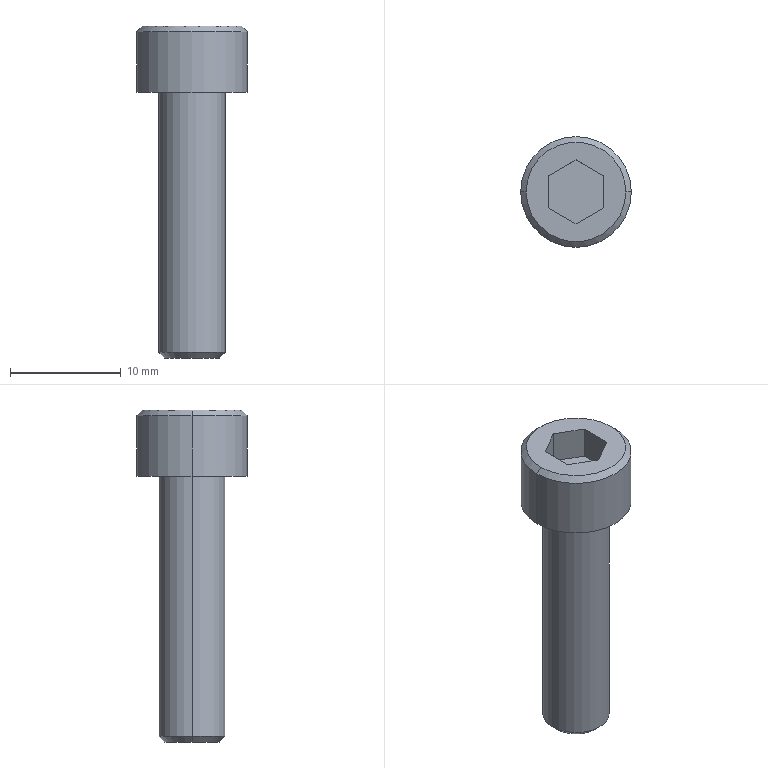Part | Creo | 1 solid | 18 faces | box 10 x 10 x 30 mm | volume 1079 mm3 | plane 10 | cone 4 | cylinder 4 | commonest cylinder face diameters 6 x2 10 x2
STEP:
#1=CARTESIAN_POINT('',(-249.5,50.,-22.));
#2=VERTEX_POINT('',#1);
#3=CARTESIAN_POINT('',(-244.5,50.,-22.));
#4=VERTEX_POINT('',#3);
#5=CARTESIAN_POINT('',(-247.,50.,-22.));
#6=DIRECTION('',(0.,0.,-1.));
#7=DIRECTION('',(-1.,0.,0.));
#8=AXIS2_PLACEMENT_3D('',#5,#6,#7);
#9=CIRCLE('',#8,2.5);
#10=EDGE_CURVE('',#2,#4,#9,.T.);
#11=ORIENTED_EDGE('',*,*,#10,.F.);
#12=CARTESIAN_POINT('',(-247.,50.,-22.));
#13=DIRECTION('',(0.,0.,-1.));
#14=DIRECTION('',(1.,0.,0.));
#15=AXIS2_PLACEMENT_3D('',#12,#13,#14);
#16=CIRCLE('',#15,2.5);
#17=EDGE_CURVE('',#4,#2,#16,.T.);
#18=ORIENTED_EDGE('',*,*,#17,.F.);
#19=EDGE_LOOP('',(#11,#18));
#20=FACE_OUTER_BOUND('',#19,.F.);
#21=CARTESIAN_POINT('',(-247.,50.,-22.));
#22=DIRECTION('',(0.,0.,-1.));
#23=DIRECTION('',(-1.,0.,0.));
#24=AXIS2_PLACEMENT_3D('',#21,#22,#23);
#25=PLANE('',#24);
#26=ADVANCED_FACE('',(#20),#25,.T.);
#27=ORIENTED_EDGE('',*,*,#10,.T.);
#28=CARTESIAN_POINT('',(-244.,50.,-21.5));
#29=VERTEX_POINT('',#28);
#30=CARTESIAN_POINT('',(-244.5,50.,-22.));
#31=DIRECTION('',(0.7071,0.,0.7071));
#32=VECTOR('',#31,0.7071);
#33=LINE('',#30,#32);
#34=EDGE_CURVE('',#4,#29,#33,.T.);
#35=ORIENTED_EDGE('',*,*,#34,.T.);
#36=CARTESIAN_POINT('',(-250.,50.,-21.5));
#37=VERTEX_POINT('',#36);
#38=CARTESIAN_POINT('',(-247.,50.,-21.5));
#39=DIRECTION('',(0.,0.,-1.));
#40=DIRECTION('',(-1.,0.,0.));
#41=AXIS2_PLACEMENT_3D('',#38,#39,#40);
#42=CIRCLE('',#41,3.);
#43=EDGE_CURVE('',#37,#29,#42,.T.);
#44=ORIENTED_EDGE('',*,*,#43,.F.);
#45=CARTESIAN_POINT('',(-249.5,50.,-22.));
#46=DIRECTION('',(-0.7071,0.,0.7071));
#47=VECTOR('',#46,0.7071);
#48=LINE('',#45,#47);
#49=EDGE_CURVE('',#2,#37,#48,.T.);
#50=ORIENTED_EDGE('',*,*,#49,.F.);
#51=EDGE_LOOP('',(#27,#35,#44,#50));
#52=FACE_OUTER_BOUND('',#51,.F.);
#53=CARTESIAN_POINT('',(-247.,50.,-21.75));
#54=DIRECTION('',(0.,0.,1.));
#55=DIRECTION('',(1.,0.,0.));
#56=AXIS2_PLACEMENT_3D('',#53,#54,#55);
#57=CONICAL_SURFACE('',#56,2.75,45.);
#58=ADVANCED_FACE('',(#52),#57,.T.);
#59=ORIENTED_EDGE('',*,*,#17,.T.);
#60=ORIENTED_EDGE('',*,*,#49,.T.);
#61=CARTESIAN_POINT('',(-247.,50.,-21.5));
#62=DIRECTION('',(0.,0.,-1.));
#63=DIRECTION('',(1.,0.,0.));
#64=AXIS2_PLACEMENT_3D('',#61,#62,#63);
#65=CIRCLE('',#64,3.);
#66=EDGE_CURVE('',#29,#37,#65,.T.);
#67=ORIENTED_EDGE('',*,*,#66,.F.);
#68=ORIENTED_EDGE('',*,*,#34,.F.);
#69=EDGE_LOOP('',(#59,#60,#67,#68));
#70=FACE_OUTER_BOUND('',#69,.F.);
#71=CARTESIAN_POINT('',(-247.,50.,-21.75));
#72=DIRECTION('',(0.,0.,1.));
#73=DIRECTION('',(1.,0.,0.));
#74=AXIS2_PLACEMENT_3D('',#71,#72,#73);
#75=CONICAL_SURFACE('',#74,2.75,45.);
#76=ADVANCED_FACE('',(#70),#75,.T.);
#77=ORIENTED_EDGE('',*,*,#66,.T.);
#78=CARTESIAN_POINT('',(-250.,50.,2.));
#79=VERTEX_POINT('',#78);
#80=CARTESIAN_POINT('',(-250.,50.,2.));
#81=DIRECTION('',(0.,0.,-1.));
#82=VECTOR('',#81,23.5);
#83=LINE('',#80,#82);
#84=EDGE_CURVE('',#79,#37,#83,.T.);
#85=ORIENTED_EDGE('',*,*,#84,.F.);
#86=CARTESIAN_POINT('',(-244.,50.,2.));
#87=VERTEX_POINT('',#86);
#88=CARTESIAN_POINT('',(-247.,50.,2.));
#89=DIRECTION('',(0.,0.,1.));
#90=DIRECTION('',(-1.,0.,0.));
#91=AXIS2_PLACEMENT_3D('',#88,#89,#90);
#92=CIRCLE('',#91,3.);
#93=EDGE_CURVE('',#79,#87,#92,.T.);
#94=ORIENTED_EDGE('',*,*,#93,.T.);
#95=CARTESIAN_POINT('',(-244.,50.,2.));
#96=DIRECTION('',(0.,0.,-1.));
#97=VECTOR('',#96,23.5);
#98=LINE('',#95,#97);
#99=EDGE_CURVE('',#87,#29,#98,.T.);
#100=ORIENTED_EDGE('',*,*,#99,.T.);
#101=EDGE_LOOP('',(#77,#85,#94,#100));
#102=FACE_OUTER_BOUND('',#101,.F.);
#103=CARTESIAN_POINT('',(-247.,50.,2.));
#104=DIRECTION('',(0.,0.,-1.));
#105=DIRECTION('',(-1.,0.,0.));
#106=AXIS2_PLACEMENT_3D('',#103,#104,#105);
#107=CYLINDRICAL_SURFACE('',#106,3.);
#108=ADVANCED_FACE('',(#102),#107,.T.);
#109=ORIENTED_EDGE('',*,*,#43,.T.);
#110=ORIENTED_EDGE('',*,*,#99,.F.);
#111=CARTESIAN_POINT('',(-247.,50.,2.));
#112=DIRECTION('',(0.,0.,1.));
#113=DIRECTION('',(1.,0.,0.));
#114=AXIS2_PLACEMENT_3D('',#111,#112,#113);
#115=CIRCLE('',#114,3.);
#116=EDGE_CURVE('',#87,#79,#115,.T.);
#117=ORIENTED_EDGE('',*,*,#116,.T.);
#118=ORIENTED_EDGE('',*,*,#84,.T.);
#119=EDGE_LOOP('',(#109,#110,#117,#118));
#120=FACE_OUTER_BOUND('',#119,.F.);
#121=CARTESIAN_POINT('',(-247.,50.,2.));
#122=DIRECTION('',(0.,0.,-1.));
#123=DIRECTION('',(-1.,0.,0.));
#124=AXIS2_PLACEMENT_3D('',#121,#122,#123);
#125=CYLINDRICAL_SURFACE('',#124,3.);
#126=ADVANCED_FACE('',(#120),#125,.T.);
#127=CARTESIAN_POINT('',(-242.,50.,2.));
#128=VERTEX_POINT('',#127);
#129=CARTESIAN_POINT('',(-252.,50.,2.));
#130=VERTEX_POINT('',#129);
#131=CARTESIAN_POINT('',(-247.,50.,2.));
#132=DIRECTION('',(0.,0.,-1.));
#133=DIRECTION('',(1.,0.,0.));
#134=AXIS2_PLACEMENT_3D('',#131,#132,#133);
#135=CIRCLE('',#134,5.);
#136=EDGE_CURVE('',#128,#130,#135,.T.);
#137=ORIENTED_EDGE('',*,*,#136,.F.);
#138=CARTESIAN_POINT('',(-247.,50.,2.));
#139=DIRECTION('',(0.,0.,-1.));
#140=DIRECTION('',(-1.,0.,0.));
#141=AXIS2_PLACEMENT_3D('',#138,#139,#140);
#142=CIRCLE('',#141,5.);
#143=EDGE_CURVE('',#130,#128,#142,.T.);
#144=ORIENTED_EDGE('',*,*,#143,.F.);
#145=EDGE_LOOP('',(#137,#144));
#146=FACE_OUTER_BOUND('',#145,.F.);
#147=ORIENTED_EDGE('',*,*,#93,.F.);
#148=ORIENTED_EDGE('',*,*,#116,.F.);
#149=EDGE_LOOP('',(#147,#148));
#150=FACE_BOUND('',#149,.F.);
#151=CARTESIAN_POINT('',(-247.,50.,2.));
#152=DIRECTION('',(0.,0.,-1.));
#153=DIRECTION('',(-1.,0.,0.));
#154=AXIS2_PLACEMENT_3D('',#151,#152,#153);
#155=PLANE('',#154);
#156=ADVANCED_FACE('',(#146,#150),#155,.T.);
#157=CARTESIAN_POINT('',(-252.,50.,7.5));
#158=VERTEX_POINT('',#157);
#159=CARTESIAN_POINT('',(-242.,50.,7.5));
#160=VERTEX_POINT('',#159);
#161=CARTESIAN_POINT('',(-247.,50.,7.5));
#162=DIRECTION('',(0.,0.,1.));
#163=DIRECTION('',(-1.,0.,0.));
#164=AXIS2_PLACEMENT_3D('',#161,#162,#163);
#165=CIRCLE('',#164,5.);
#166=EDGE_CURVE('',#158,#160,#165,.T.);
#167=ORIENTED_EDGE('',*,*,#166,.T.);
#168=CARTESIAN_POINT('',(-242.,50.,2.));
#169=DIRECTION('',(0.,0.,1.));
#170=VECTOR('',#169,5.5);
#171=LINE('',#168,#170);
#172=EDGE_CURVE('',#128,#160,#171,.T.);
#173=ORIENTED_EDGE('',*,*,#172,.F.);
#174=ORIENTED_EDGE('',*,*,#136,.T.);
#175=CARTESIAN_POINT('',(-252.,50.,2.));
#176=DIRECTION('',(0.,0.,1.));
#177=VECTOR('',#176,5.5);
#178=LINE('',#175,#177);
#179=EDGE_CURVE('',#130,#158,#178,.T.);
#180=ORIENTED_EDGE('',*,*,#179,.T.);
#181=EDGE_LOOP('',(#167,#173,#174,#180));
#182=FACE_OUTER_BOUND('',#181,.F.);
#183=CARTESIAN_POINT('',(-247.,50.,2.));
#184=DIRECTION('',(0.,0.,1.));
#185=DIRECTION('',(1.,0.,0.));
#186=AXIS2_PLACEMENT_3D('',#183,#184,#185);
#187=CYLINDRICAL_SURFACE('',#186,5.);
#188=ADVANCED_FACE('',(#182),#187,.T.);
#189=CARTESIAN_POINT('',(-251.5,50.,8.));
#190=VERTEX_POINT('',#189);
#191=CARTESIAN_POINT('',(-242.5,50.,8.));
#192=VERTEX_POINT('',#191);
#193=CARTESIAN_POINT('',(-247.,50.,8.));
#194=DIRECTION('',(0.,0.,1.));
#195=DIRECTION('',(-1.,0.,0.));
#196=AXIS2_PLACEMENT_3D('',#193,#194,#195);
#197=CIRCLE('',#196,4.5);
#198=EDGE_CURVE('',#190,#192,#197,.T.);
#199=ORIENTED_EDGE('',*,*,#198,.T.);
#200=CARTESIAN_POINT('',(-242.5,50.,8.));
#201=DIRECTION('',(0.7071,0.,-0.7071));
#202=VECTOR('',#201,0.7071);
#203=LINE('',#200,#202);
#204=EDGE_CURVE('',#192,#160,#203,.T.);
#205=ORIENTED_EDGE('',*,*,#204,.T.);
#206=ORIENTED_EDGE('',*,*,#166,.F.);
#207=CARTESIAN_POINT('',(-251.5,50.,8.));
#208=DIRECTION('',(-0.7071,0.,-0.7071));
#209=VECTOR('',#208,0.7071);
#210=LINE('',#207,#209);
#211=EDGE_CURVE('',#190,#158,#210,.T.);
#212=ORIENTED_EDGE('',*,*,#211,.F.);
#213=EDGE_LOOP('',(#199,#205,#206,#212));
#214=FACE_OUTER_BOUND('',#213,.F.);
#215=CARTESIAN_POINT('',(-247.,50.,7.75));
#216=DIRECTION('',(0.,0.,-1.));
#217=DIRECTION('',(-1.,0.,0.));
#218=AXIS2_PLACEMENT_3D('',#215,#216,#217);
#219=CONICAL_SURFACE('',#218,4.75,45.);
#220=ADVANCED_FACE('',(#214),#219,.T.);
#221=CARTESIAN_POINT('',(-247.,50.,8.));
#222=DIRECTION('',(0.,0.,1.));
#223=DIRECTION('',(1.,0.,0.));
#224=AXIS2_PLACEMENT_3D('',#221,#222,#223);
#225=CIRCLE('',#224,4.5);
#226=EDGE_CURVE('',#192,#190,#225,.T.);
#227=ORIENTED_EDGE('',*,*,#226,.F.);
#228=ORIENTED_EDGE('',*,*,#198,.F.);
#229=EDGE_LOOP('',(#227,#228));
#230=FACE_OUTER_BOUND('',#229,.F.);
#231=CARTESIAN_POINT('',(-249.5,48.557,8.));
#232=VERTEX_POINT('',#231);
#233=CARTESIAN_POINT('',(-249.5,51.443,8.));
#234=VERTEX_POINT('',#233);
#235=CARTESIAN_POINT('',(-249.5,48.557,8.));
#236=DIRECTION('',(0.,1.,0.));
#237=VECTOR('',#236,2.887);
#238=LINE('',#235,#237);
#239=EDGE_CURVE('',#232,#234,#238,.T.);
#240=ORIENTED_EDGE('',*,*,#239,.F.);
#241=CARTESIAN_POINT('',(-247.,47.113,8.));
#242=VERTEX_POINT('',#241);
#243=CARTESIAN_POINT('',(-247.,47.113,8.));
#244=DIRECTION('',(-0.866,0.5,0.));
#245=VECTOR('',#244,2.887);
#246=LINE('',#243,#245);
#247=EDGE_CURVE('',#242,#232,#246,.T.);
#248=ORIENTED_EDGE('',*,*,#247,.F.);
#249=CARTESIAN_POINT('',(-244.5,48.557,8.));
#250=VERTEX_POINT('',#249);
#251=CARTESIAN_POINT('',(-244.5,48.557,8.));
#252=DIRECTION('',(-0.866,-0.5,0.));
#253=VECTOR('',#252,2.887);
#254=LINE('',#251,#253);
#255=EDGE_CURVE('',#250,#242,#254,.T.);
#256=ORIENTED_EDGE('',*,*,#255,.F.);
#257=CARTESIAN_POINT('',(-244.5,51.443,8.));
#258=VERTEX_POINT('',#257);
#259=CARTESIAN_POINT('',(-244.5,51.443,8.));
#260=DIRECTION('',(0.,-1.,0.));
#261=VECTOR('',#260,2.887);
#262=LINE('',#259,#261);
#263=EDGE_CURVE('',#258,#250,#262,.T.);
#264=ORIENTED_EDGE('',*,*,#263,.F.);
#265=CARTESIAN_POINT('',(-247.,52.887,8.));
#266=VERTEX_POINT('',#265);
#267=CARTESIAN_POINT('',(-247.,52.887,8.));
#268=DIRECTION('',(0.866,-0.5,0.));
#269=VECTOR('',#268,2.887);
#270=LINE('',#267,#269);
#271=EDGE_CURVE('',#266,#258,#270,.T.);
#272=ORIENTED_EDGE('',*,*,#271,.F.);
#273=CARTESIAN_POINT('',(-249.5,51.443,8.));
#274=DIRECTION('',(0.866,0.5,0.));
#275=VECTOR('',#274,2.887);
#276=LINE('',#273,#275);
#277=EDGE_CURVE('',#234,#266,#276,.T.);
#278=ORIENTED_EDGE('',*,*,#277,.F.);
#279=EDGE_LOOP('',(#240,#248,#256,#264,#272,#278));
#280=FACE_BOUND('',#279,.F.);
#281=CARTESIAN_POINT('',(-247.,50.,8.));
#282=DIRECTION('',(0.,0.,1.));
#283=DIRECTION('',(1.,0.,0.));
#284=AXIS2_PLACEMENT_3D('',#281,#282,#283);
#285=PLANE('',#284);
#286=ADVANCED_FACE('',(#230,#280),#285,.T.);
#287=ORIENTED_EDGE('',*,*,#226,.T.);
#288=ORIENTED_EDGE('',*,*,#211,.T.);
#289=CARTESIAN_POINT('',(-247.,50.,7.5));
#290=DIRECTION('',(0.,0.,1.));
#291=DIRECTION('',(1.,0.,0.));
#292=AXIS2_PLACEMENT_3D('',#289,#290,#291);
#293=CIRCLE('',#292,5.);
#294=EDGE_CURVE('',#160,#158,#293,.T.);
#295=ORIENTED_EDGE('',*,*,#294,.F.);
#296=ORIENTED_EDGE('',*,*,#204,.F.);
#297=EDGE_LOOP('',(#287,#288,#295,#296));
#298=FACE_OUTER_BOUND('',#297,.F.);
#299=CARTESIAN_POINT('',(-247.,50.,7.75));
#300=DIRECTION('',(0.,0.,-1.));
#301=DIRECTION('',(-1.,0.,0.));
#302=AXIS2_PLACEMENT_3D('',#299,#300,#301);
#303=CONICAL_SURFACE('',#302,4.75,45.);
#304=ADVANCED_FACE('',(#298),#303,.T.);
#305=ORIENTED_EDGE('',*,*,#294,.T.);
#306=ORIENTED_EDGE('',*,*,#179,.F.);
#307=ORIENTED_EDGE('',*,*,#143,.T.);
#308=ORIENTED_EDGE('',*,*,#172,.T.);
#309=EDGE_LOOP('',(#305,#306,#307,#308));
#310=FACE_OUTER_BOUND('',#309,.F.);
#311=CARTESIAN_POINT('',(-247.,50.,2.));
#312=DIRECTION('',(0.,0.,1.));
#313=DIRECTION('',(1.,0.,0.));
#314=AXIS2_PLACEMENT_3D('',#311,#312,#313);
#315=CYLINDRICAL_SURFACE('',#314,5.);
#316=ADVANCED_FACE('',(#310),#315,.T.);
#317=ORIENTED_EDGE('',*,*,#239,.T.);
#318=CARTESIAN_POINT('',(-249.5,51.443,5.));
#319=VERTEX_POINT('',#318);
#320=CARTESIAN_POINT('',(-249.5,51.443,8.));
#321=DIRECTION('',(0.,0.,-1.));
#322=VECTOR('',#321,3.);
#323=LINE('',#320,#322);
#324=EDGE_CURVE('',#234,#319,#323,.T.);
#325=ORIENTED_EDGE('',*,*,#324,.T.);
#326=CARTESIAN_POINT('',(-249.5,48.557,5.));
#327=VERTEX_POINT('',#326);
#328=CARTESIAN_POINT('',(-249.5,48.557,5.));
#329=DIRECTION('',(0.,1.,0.));
#330=VECTOR('',#329,2.887);
#331=LINE('',#328,#330);
#332=EDGE_CURVE('',#327,#319,#331,.T.);
#333=ORIENTED_EDGE('',*,*,#332,.F.);
#334=CARTESIAN_POINT('',(-249.5,48.557,8.));
#335=DIRECTION('',(0.,0.,-1.));
#336=VECTOR('',#335,3.);
#337=LINE('',#334,#336);
#338=EDGE_CURVE('',#232,#327,#337,.T.);
#339=ORIENTED_EDGE('',*,*,#338,.F.);
#340=EDGE_LOOP('',(#317,#325,#333,#339));
#341=FACE_OUTER_BOUND('',#340,.F.);
#342=CARTESIAN_POINT('',(-249.5,50.,6.5));
#343=DIRECTION('',(-1.,0.,0.));
#344=DIRECTION('',(0.,0.,1.));
#345=AXIS2_PLACEMENT_3D('',#342,#343,#344);
#346=PLANE('',#345);
#347=ADVANCED_FACE('',(#341),#346,.F.);
#348=ORIENTED_EDGE('',*,*,#277,.T.);
#349=CARTESIAN_POINT('',(-247.,52.887,5.));
#350=VERTEX_POINT('',#349);
#351=CARTESIAN_POINT('',(-247.,52.887,8.));
#352=DIRECTION('',(0.,0.,-1.));
#353=VECTOR('',#352,3.);
#354=LINE('',#351,#353);
#355=EDGE_CURVE('',#266,#350,#354,.T.);
#356=ORIENTED_EDGE('',*,*,#355,.T.);
#357=CARTESIAN_POINT('',(-247.,52.887,5.));
#358=DIRECTION('',(-0.866,-0.5,0.));
#359=VECTOR('',#358,2.887);
#360=LINE('',#357,#359);
#361=EDGE_CURVE('',#350,#319,#360,.T.);
#362=ORIENTED_EDGE('',*,*,#361,.T.);
#363=ORIENTED_EDGE('',*,*,#324,.F.);
#364=EDGE_LOOP('',(#348,#356,#362,#363));
#365=FACE_OUTER_BOUND('',#364,.F.);
#366=CARTESIAN_POINT('',(-248.25,52.165,6.5));
#367=DIRECTION('',(-0.5,0.866,0.));
#368=DIRECTION('',(-0.866,-0.5,0.));
#369=AXIS2_PLACEMENT_3D('',#366,#367,#368);
#370=PLANE('',#369);
#371=ADVANCED_FACE('',(#365),#370,.F.);
#372=ORIENTED_EDGE('',*,*,#271,.T.);
#373=CARTESIAN_POINT('',(-244.5,51.443,5.));
#374=VERTEX_POINT('',#373);
#375=CARTESIAN_POINT('',(-244.5,51.443,8.));
#376=DIRECTION('',(0.,0.,-1.));
#377=VECTOR('',#376,3.);
#378=LINE('',#375,#377);
#379=EDGE_CURVE('',#258,#374,#378,.T.);
#380=ORIENTED_EDGE('',*,*,#379,.T.);
#381=CARTESIAN_POINT('',(-244.5,51.443,5.));
#382=DIRECTION('',(-0.866,0.5,0.));
#383=VECTOR('',#382,2.887);
#384=LINE('',#381,#383);
#385=EDGE_CURVE('',#374,#350,#384,.T.);
#386=ORIENTED_EDGE('',*,*,#385,.T.);
#387=ORIENTED_EDGE('',*,*,#355,.F.);
#388=EDGE_LOOP('',(#372,#380,#386,#387));
#389=FACE_OUTER_BOUND('',#388,.F.);
#390=CARTESIAN_POINT('',(-245.75,52.165,6.5));
#391=DIRECTION('',(0.5,0.866,0.));
#392=DIRECTION('',(-0.866,0.5,0.));
#393=AXIS2_PLACEMENT_3D('',#390,#391,#392);
#394=PLANE('',#393);
#395=ADVANCED_FACE('',(#389),#394,.F.);
#396=ORIENTED_EDGE('',*,*,#263,.T.);
#397=CARTESIAN_POINT('',(-244.5,48.557,5.));
#398=VERTEX_POINT('',#397);
#399=CARTESIAN_POINT('',(-244.5,48.557,8.));
#400=DIRECTION('',(0.,0.,-1.));
#401=VECTOR('',#400,3.);
#402=LINE('',#399,#401);
#403=EDGE_CURVE('',#250,#398,#402,.T.);
#404=ORIENTED_EDGE('',*,*,#403,.T.);
#405=CARTESIAN_POINT('',(-244.5,51.443,5.));
#406=DIRECTION('',(0.,-1.,0.));
#407=VECTOR('',#406,2.887);
#408=LINE('',#405,#407);
#409=EDGE_CURVE('',#374,#398,#408,.T.);
#410=ORIENTED_EDGE('',*,*,#409,.F.);
#411=ORIENTED_EDGE('',*,*,#379,.F.);
#412=EDGE_LOOP('',(#396,#404,#410,#411));
#413=FACE_OUTER_BOUND('',#412,.F.);
#414=CARTESIAN_POINT('',(-244.5,50.,6.5));
#415=DIRECTION('',(1.,0.,0.));
#416=DIRECTION('',(0.,0.,-1.));
#417=AXIS2_PLACEMENT_3D('',#414,#415,#416);
#418=PLANE('',#417);
#419=ADVANCED_FACE('',(#413),#418,.F.);
#420=ORIENTED_EDGE('',*,*,#255,.T.);
#421=CARTESIAN_POINT('',(-247.,47.113,5.));
#422=VERTEX_POINT('',#421);
#423=CARTESIAN_POINT('',(-247.,47.113,8.));
#424=DIRECTION('',(0.,0.,-1.));
#425=VECTOR('',#424,3.);
#426=LINE('',#423,#425);
#427=EDGE_CURVE('',#242,#422,#426,.T.);
#428=ORIENTED_EDGE('',*,*,#427,.T.);
#429=CARTESIAN_POINT('',(-247.,47.113,5.));
#430=DIRECTION('',(0.866,0.5,0.));
#431=VECTOR('',#430,2.887);
#432=LINE('',#429,#431);
#433=EDGE_CURVE('',#422,#398,#432,.T.);
#434=ORIENTED_EDGE('',*,*,#433,.T.);
#435=ORIENTED_EDGE('',*,*,#403,.F.);
#436=EDGE_LOOP('',(#420,#428,#434,#435));
#437=FACE_OUTER_BOUND('',#436,.F.);
#438=CARTESIAN_POINT('',(-245.75,47.835,6.5));
#439=DIRECTION('',(0.5,-0.866,0.));
#440=DIRECTION('',(0.866,0.5,0.));
#441=AXIS2_PLACEMENT_3D('',#438,#439,#440);
#442=PLANE('',#441);
#443=ADVANCED_FACE('',(#437),#442,.F.);
#444=ORIENTED_EDGE('',*,*,#247,.T.);
#445=ORIENTED_EDGE('',*,*,#338,.T.);
#446=CARTESIAN_POINT('',(-249.5,48.557,5.));
#447=DIRECTION('',(0.866,-0.5,0.));
#448=VECTOR('',#447,2.887);
#449=LINE('',#446,#448);
#450=EDGE_CURVE('',#327,#422,#449,.T.);
#451=ORIENTED_EDGE('',*,*,#450,.T.);
#452=ORIENTED_EDGE('',*,*,#427,.F.);
#453=EDGE_LOOP('',(#444,#445,#451,#452));
#454=FACE_OUTER_BOUND('',#453,.F.);
#455=CARTESIAN_POINT('',(-248.25,47.835,6.5));
#456=DIRECTION('',(-0.5,-0.866,0.));
#457=DIRECTION('',(0.866,-0.5,0.));
#458=AXIS2_PLACEMENT_3D('',#455,#456,#457);
#459=PLANE('',#458);
#460=ADVANCED_FACE('',(#454),#459,.F.);
#461=ORIENTED_EDGE('',*,*,#433,.F.);
#462=ORIENTED_EDGE('',*,*,#450,.F.);
#463=ORIENTED_EDGE('',*,*,#332,.T.);
#464=ORIENTED_EDGE('',*,*,#361,.F.);
#465=ORIENTED_EDGE('',*,*,#385,.F.);
#466=ORIENTED_EDGE('',*,*,#409,.T.);
#467=EDGE_LOOP('',(#461,#462,#463,#464,#465,#466));
#468=FACE_OUTER_BOUND('',#467,.F.);
#469=CARTESIAN_POINT('',(-247.,50.,5.));
#470=DIRECTION('',(0.,0.,-1.));
#471=DIRECTION('',(-1.,0.,0.));
#472=AXIS2_PLACEMENT_3D('',#469,#470,#471);
#473=PLANE('',#472);
#474=ADVANCED_FACE('',(#468),#473,.F.);
#475=CLOSED_SHELL('',(#26,#58,#76,#108,#126,#156,#188,#220,#286,#304,#316,#347,#371,#395,#419,#443,#460,#474));
#476=MANIFOLD_SOLID_BREP('',#475);
#477=(LENGTH_UNIT()NAMED_UNIT(*)SI_UNIT(.MILLI.,.METRE.));
#478=UNCERTAINTY_MEASURE_WITH_UNIT(LENGTH_MEASURE(0.003317),#477,'','');
#479=(NAMED_UNIT(*)PLANE_ANGLE_UNIT()SI_UNIT($,.RADIAN.));
#480=PLANE_ANGLE_MEASURE_WITH_UNIT(PLANE_ANGLE_MEASURE(0.01745),#479);
#481=(CONVERSION_BASED_UNIT('DEGREE',#480)NAMED_UNIT(*)PLANE_ANGLE_UNIT());
#482=(NAMED_UNIT(*)SI_UNIT($,.STERADIAN.)SOLID_ANGLE_UNIT());
#483=(GEOMETRIC_REPRESENTATION_CONTEXT(3)GLOBAL_UNCERTAINTY_ASSIGNED_CONTEXT((#478))GLOBAL_UNIT_ASSIGNED_CONTEXT((#477,#481,#482))REPRESENTATION_CONTEXT('',''));
#484=ADVANCED_BREP_SHAPE_REPRESENTATION('',(#476),#483);